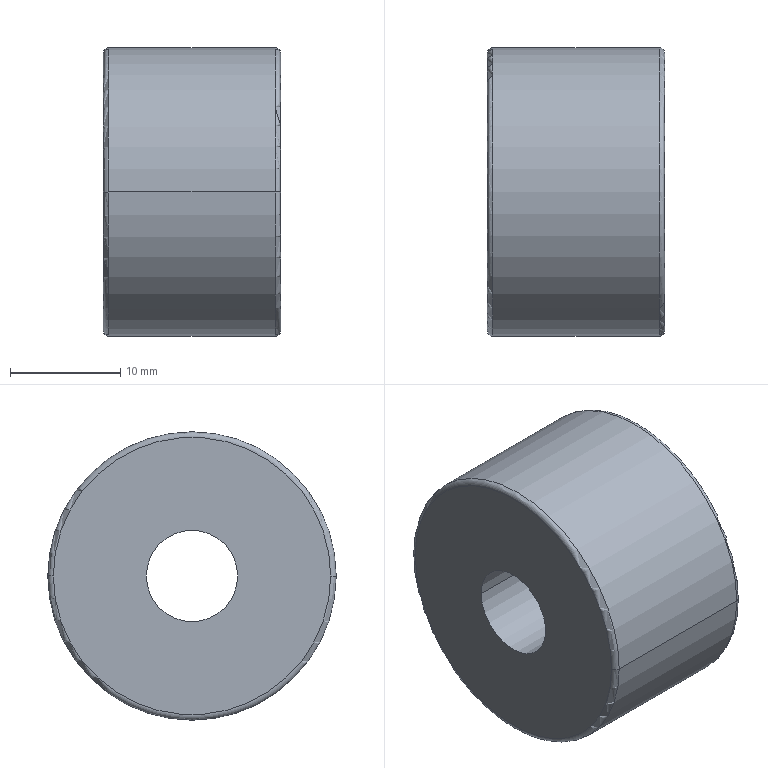Part | STEP file | 8XS224021_8GD.211.061 | 1 solid | 10 faces | box 16.1 x 26.2 x 26.2 mm | volume 7800 mm3 | torus 4 | cylinder 4 | plane 2 | commonest cylinder face diameters 8.3 x2 26.2 x2
STEP:
#1=CARTESIAN_POINT('',(0.,0.,0.));
#2=DIRECTION('',(0.,0.,1.));
#3=DIRECTION('',(1.,0.,0.));
#4=AXIS2_PLACEMENT_3D('',#1,#2,#3);
#5=CARTESIAN_POINT('',(5.5,-13.1,0.));
#6=VERTEX_POINT('',#5);
#7=CARTESIAN_POINT('',(5.5,13.1,0.));
#8=VERTEX_POINT('',#7);
#9=CARTESIAN_POINT('',(5.5,0.,0.));
#10=DIRECTION('',(-1.,0.,0.));
#11=DIRECTION('',(0.,1.,0.));
#12=AXIS2_PLACEMENT_3D('',#9,#10,#11);
#13=CIRCLE('',#12,13.1);
#14=CARTESIAN_POINT('',(5.5,0.,0.));
#15=DIRECTION('',(1.,0.,0.));
#16=DIRECTION('',(0.,1.,0.));
#17=AXIS2_PLACEMENT_3D('',#14,#15,#16);
#18=TOROIDAL_SURFACE('',#17,12.6,0.5);
#19=CARTESIAN_POINT('',(6.283,0.));
#20=DIRECTION('',(-1.,0.));
#21=VECTOR('',#20,1.);
#22=LINE('',#19,#21);
#23=(GEOMETRIC_REPRESENTATION_CONTEXT(2)PARAMETRIC_REPRESENTATION_CONTEXT()REPRESENTATION_CONTEXT('',''));
#24=DEFINITIONAL_REPRESENTATION('',(#22),#23);
#25=PCURVE('',#18,#24);
#26=CARTESIAN_POINT('',(6.,0.,0.));
#27=DIRECTION('',(1.,0.,0.));
#28=DIRECTION('',(0.,1.,0.));
#29=AXIS2_PLACEMENT_3D('',#26,#27,#28);
#30=CYLINDRICAL_SURFACE('',#29,13.1);
#31=CARTESIAN_POINT('',(6.283,-0.5));
#32=DIRECTION('',(-1.,0.));
#33=VECTOR('',#32,1.);
#34=LINE('',#31,#33);
#35=(GEOMETRIC_REPRESENTATION_CONTEXT(2)PARAMETRIC_REPRESENTATION_CONTEXT()REPRESENTATION_CONTEXT('',''));
#36=DEFINITIONAL_REPRESENTATION('',(#34),#35);
#37=PCURVE('',#30,#36);
#38=SURFACE_CURVE('',#13,(#25,#37),.PCURVE_S1.);
#39=EDGE_CURVE('',#6,#8,#38,.T.);
#40=ORIENTED_EDGE('',*,*,#39,.F.);
#41=CARTESIAN_POINT('',(6.,-12.6,0.));
#42=VERTEX_POINT('',#41);
#43=CARTESIAN_POINT('',(5.5,-12.6,0.));
#44=DIRECTION('',(0.,0.,1.));
#45=DIRECTION('',(0.,-1.,0.));
#46=AXIS2_PLACEMENT_3D('',#43,#44,#45);
#47=CIRCLE('',#46,0.5);
#48=CARTESIAN_POINT('',(3.142,0.));
#49=DIRECTION('',(0.,1.));
#50=VECTOR('',#49,1.);
#51=LINE('',#48,#50);
#52=(GEOMETRIC_REPRESENTATION_CONTEXT(2)PARAMETRIC_REPRESENTATION_CONTEXT()REPRESENTATION_CONTEXT('',''));
#53=DEFINITIONAL_REPRESENTATION('',(#51),#52);
#54=PCURVE('',#18,#53);
#55=CARTESIAN_POINT('',(5.5,0.,0.));
#56=DIRECTION('',(1.,0.,0.));
#57=DIRECTION('',(0.,1.,0.));
#58=AXIS2_PLACEMENT_3D('',#55,#56,#57);
#59=TOROIDAL_SURFACE('',#58,12.6,0.5);
#60=CARTESIAN_POINT('',(3.142,0.));
#61=DIRECTION('',(0.,1.));
#62=VECTOR('',#61,1.);
#63=LINE('',#60,#62);
#64=(GEOMETRIC_REPRESENTATION_CONTEXT(2)PARAMETRIC_REPRESENTATION_CONTEXT()REPRESENTATION_CONTEXT('',''));
#65=DEFINITIONAL_REPRESENTATION('',(#63),#64);
#66=PCURVE('',#59,#65);
#67=SURFACE_CURVE('',#47,(#54,#66),.PCURVE_S1.);
#68=EDGE_CURVE('',#6,#42,#67,.T.);
#69=ORIENTED_EDGE('',*,*,#68,.T.);
#70=CARTESIAN_POINT('',(6.,12.6,0.));
#71=VERTEX_POINT('',#70);
#72=CARTESIAN_POINT('',(6.,0.,0.));
#73=DIRECTION('',(1.,0.,0.));
#74=DIRECTION('',(0.,1.,0.));
#75=AXIS2_PLACEMENT_3D('',#72,#73,#74);
#76=CIRCLE('',#75,12.6);
#77=CARTESIAN_POINT('',(0.,1.571));
#78=DIRECTION('',(1.,0.));
#79=VECTOR('',#78,1.);
#80=LINE('',#77,#79);
#81=(GEOMETRIC_REPRESENTATION_CONTEXT(2)PARAMETRIC_REPRESENTATION_CONTEXT()REPRESENTATION_CONTEXT('',''));
#82=DEFINITIONAL_REPRESENTATION('',(#80),#81);
#83=PCURVE('',#18,#82);
#84=CARTESIAN_POINT('',(6.,13.1,0.));
#85=DIRECTION('',(1.,0.,0.));
#86=DIRECTION('',(0.,1.,0.));
#87=AXIS2_PLACEMENT_3D('',#84,#85,#86);
#88=PLANE('',#87);
#89=CARTESIAN_POINT('',(-13.1,0.));
#90=DIRECTION('',(1.,0.));
#91=AXIS2_PLACEMENT_2D('',#89,#90);
#92=CIRCLE('',#91,12.6);
#93=(GEOMETRIC_REPRESENTATION_CONTEXT(2)PARAMETRIC_REPRESENTATION_CONTEXT()REPRESENTATION_CONTEXT('',''));
#94=DEFINITIONAL_REPRESENTATION('',(#92),#93);
#95=PCURVE('',#88,#94);
#96=SURFACE_CURVE('',#76,(#83,#95),.PCURVE_S1.);
#97=EDGE_CURVE('',#71,#42,#96,.T.);
#98=ORIENTED_EDGE('',*,*,#97,.F.);
#99=CARTESIAN_POINT('',(5.5,12.6,0.));
#100=DIRECTION('',(0.,0.,-1.));
#101=DIRECTION('',(-1.,0.,0.));
#102=AXIS2_PLACEMENT_3D('',#99,#100,#101);
#103=CIRCLE('',#102,0.5);
#104=CARTESIAN_POINT('',(0.,-1.571));
#105=DIRECTION('',(0.,1.));
#106=VECTOR('',#105,1.);
#107=LINE('',#104,#106);
#108=(GEOMETRIC_REPRESENTATION_CONTEXT(2)PARAMETRIC_REPRESENTATION_CONTEXT()REPRESENTATION_CONTEXT('',''));
#109=DEFINITIONAL_REPRESENTATION('',(#107),#108);
#110=PCURVE('',#18,#109);
#111=CARTESIAN_POINT('',(6.283,-1.571));
#112=DIRECTION('',(0.,1.));
#113=VECTOR('',#112,1.);
#114=LINE('',#111,#113);
#115=(GEOMETRIC_REPRESENTATION_CONTEXT(2)PARAMETRIC_REPRESENTATION_CONTEXT()REPRESENTATION_CONTEXT('',''));
#116=DEFINITIONAL_REPRESENTATION('',(#114),#115);
#117=PCURVE('',#59,#116);
#118=SURFACE_CURVE('',#103,(#110,#117),.PCURVE_S1.);
#119=EDGE_CURVE('',#8,#71,#118,.T.);
#120=ORIENTED_EDGE('',*,*,#119,.F.);
#121=EDGE_LOOP('',(#40,#69,#98,#120));
#122=FACE_BOUND('',#121,.T.);
#123=ADVANCED_FACE('',(#122),#18,.T.);
#124=CARTESIAN_POINT('',(-9.6,13.1,0.));
#125=VERTEX_POINT('',#124);
#126=CARTESIAN_POINT('',(-9.6,-13.1,0.));
#127=VERTEX_POINT('',#126);
#128=CARTESIAN_POINT('',(-9.6,0.,0.));
#129=DIRECTION('',(1.,0.,0.));
#130=DIRECTION('',(0.,-1.,0.));
#131=AXIS2_PLACEMENT_3D('',#128,#129,#130);
#132=CIRCLE('',#131,13.1);
#133=CARTESIAN_POINT('',(-9.6,0.,0.));
#134=DIRECTION('',(-1.,0.,0.));
#135=DIRECTION('',(0.,-1.,0.));
#136=AXIS2_PLACEMENT_3D('',#133,#134,#135);
#137=TOROIDAL_SURFACE('',#136,12.6,0.5);
#138=CARTESIAN_POINT('',(6.283,0.));
#139=DIRECTION('',(-1.,0.));
#140=VECTOR('',#139,1.);
#141=LINE('',#138,#140);
#142=(GEOMETRIC_REPRESENTATION_CONTEXT(2)PARAMETRIC_REPRESENTATION_CONTEXT()REPRESENTATION_CONTEXT('',''));
#143=DEFINITIONAL_REPRESENTATION('',(#141),#142);
#144=PCURVE('',#137,#143);
#145=CARTESIAN_POINT('',(-3.142,-15.6));
#146=DIRECTION('',(1.,0.));
#147=VECTOR('',#146,1.);
#148=LINE('',#145,#147);
#149=(GEOMETRIC_REPRESENTATION_CONTEXT(2)PARAMETRIC_REPRESENTATION_CONTEXT()REPRESENTATION_CONTEXT('',''));
#150=DEFINITIONAL_REPRESENTATION('',(#148),#149);
#151=PCURVE('',#30,#150);
#152=SURFACE_CURVE('',#132,(#144,#151),.PCURVE_S1.);
#153=EDGE_CURVE('',#125,#127,#152,.T.);
#154=ORIENTED_EDGE('',*,*,#153,.F.);
#155=CARTESIAN_POINT('',(-10.1,12.6,0.));
#156=VERTEX_POINT('',#155);
#157=CARTESIAN_POINT('',(-9.6,12.6,0.));
#158=DIRECTION('',(0.,0.,1.));
#159=DIRECTION('',(0.,-1.,0.));
#160=AXIS2_PLACEMENT_3D('',#157,#158,#159);
#161=CIRCLE('',#160,0.5);
#162=CARTESIAN_POINT('',(3.142,-3.142));
#163=DIRECTION('',(0.,1.));
#164=VECTOR('',#163,1.);
#165=LINE('',#162,#164);
#166=(GEOMETRIC_REPRESENTATION_CONTEXT(2)PARAMETRIC_REPRESENTATION_CONTEXT()REPRESENTATION_CONTEXT('',''));
#167=DEFINITIONAL_REPRESENTATION('',(#165),#166);
#168=PCURVE('',#137,#167);
#169=CARTESIAN_POINT('',(-9.6,0.,0.));
#170=DIRECTION('',(-1.,0.,0.));
#171=DIRECTION('',(0.,-1.,0.));
#172=AXIS2_PLACEMENT_3D('',#169,#170,#171);
#173=TOROIDAL_SURFACE('',#172,12.6,0.5);
#174=CARTESIAN_POINT('',(3.142,-3.142));
#175=DIRECTION('',(0.,1.));
#176=VECTOR('',#175,1.);
#177=LINE('',#174,#176);
#178=(GEOMETRIC_REPRESENTATION_CONTEXT(2)PARAMETRIC_REPRESENTATION_CONTEXT()REPRESENTATION_CONTEXT('',''));
#179=DEFINITIONAL_REPRESENTATION('',(#177),#178);
#180=PCURVE('',#173,#179);
#181=SURFACE_CURVE('',#161,(#168,#180),.PCURVE_S1.);
#182=EDGE_CURVE('',#125,#156,#181,.T.);
#183=ORIENTED_EDGE('',*,*,#182,.T.);
#184=CARTESIAN_POINT('',(-10.1,-12.6,0.));
#185=VERTEX_POINT('',#184);
#186=CARTESIAN_POINT('',(-10.1,0.,0.));
#187=DIRECTION('',(-1.,0.,0.));
#188=DIRECTION('',(0.,-1.,0.));
#189=AXIS2_PLACEMENT_3D('',#186,#187,#188);
#190=CIRCLE('',#189,12.6);
#191=CARTESIAN_POINT('',(0.,1.571));
#192=DIRECTION('',(1.,0.));
#193=VECTOR('',#192,1.);
#194=LINE('',#191,#193);
#195=(GEOMETRIC_REPRESENTATION_CONTEXT(2)PARAMETRIC_REPRESENTATION_CONTEXT()REPRESENTATION_CONTEXT('',''));
#196=DEFINITIONAL_REPRESENTATION('',(#194),#195);
#197=PCURVE('',#137,#196);
#198=CARTESIAN_POINT('',(-10.1,13.1,0.));
#199=DIRECTION('',(-1.,0.,0.));
#200=DIRECTION('',(0.,-1.,0.));
#201=AXIS2_PLACEMENT_3D('',#198,#199,#200);
#202=PLANE('',#201);
#203=CARTESIAN_POINT('',(13.1,0.));
#204=DIRECTION('',(1.,0.));
#205=AXIS2_PLACEMENT_2D('',#203,#204);
#206=CIRCLE('',#205,12.6);
#207=(GEOMETRIC_REPRESENTATION_CONTEXT(2)PARAMETRIC_REPRESENTATION_CONTEXT()REPRESENTATION_CONTEXT('',''));
#208=DEFINITIONAL_REPRESENTATION('',(#206),#207);
#209=PCURVE('',#202,#208);
#210=SURFACE_CURVE('',#190,(#197,#209),.PCURVE_S1.);
#211=EDGE_CURVE('',#185,#156,#210,.T.);
#212=ORIENTED_EDGE('',*,*,#211,.F.);
#213=CARTESIAN_POINT('',(-9.6,-12.6,0.));
#214=DIRECTION('',(0.,0.,-1.));
#215=DIRECTION('',(-1.,0.,0.));
#216=AXIS2_PLACEMENT_3D('',#213,#214,#215);
#217=CIRCLE('',#216,0.5);
#218=CARTESIAN_POINT('',(0.,-4.712));
#219=DIRECTION('',(0.,1.));
#220=VECTOR('',#219,1.);
#221=LINE('',#218,#220);
#222=(GEOMETRIC_REPRESENTATION_CONTEXT(2)PARAMETRIC_REPRESENTATION_CONTEXT()REPRESENTATION_CONTEXT('',''));
#223=DEFINITIONAL_REPRESENTATION('',(#221),#222);
#224=PCURVE('',#137,#223);
#225=CARTESIAN_POINT('',(6.283,-4.712));
#226=DIRECTION('',(0.,1.));
#227=VECTOR('',#226,1.);
#228=LINE('',#225,#227);
#229=(GEOMETRIC_REPRESENTATION_CONTEXT(2)PARAMETRIC_REPRESENTATION_CONTEXT()REPRESENTATION_CONTEXT('',''));
#230=DEFINITIONAL_REPRESENTATION('',(#228),#229);
#231=PCURVE('',#173,#230);
#232=SURFACE_CURVE('',#217,(#224,#231),.PCURVE_S1.);
#233=EDGE_CURVE('',#127,#185,#232,.T.);
#234=ORIENTED_EDGE('',*,*,#233,.F.);
#235=EDGE_LOOP('',(#154,#183,#212,#234));
#236=FACE_BOUND('',#235,.T.);
#237=ADVANCED_FACE('',(#236),#137,.T.);
#238=ORIENTED_EDGE('',*,*,#153,.T.);
#239=CARTESIAN_POINT('',(6.,-13.1,0.));
#240=DIRECTION('',(1.,0.,0.));
#241=VECTOR('',#240,1.);
#242=LINE('',#239,#241);
#243=CARTESIAN_POINT('',(3.142,0.));
#244=DIRECTION('',(0.,1.));
#245=VECTOR('',#244,1.);
#246=LINE('',#243,#245);
#247=(GEOMETRIC_REPRESENTATION_CONTEXT(2)PARAMETRIC_REPRESENTATION_CONTEXT()REPRESENTATION_CONTEXT('',''));
#248=DEFINITIONAL_REPRESENTATION('',(#246),#247);
#249=PCURVE('',#30,#248);
#250=CARTESIAN_POINT('',(6.,0.,0.));
#251=DIRECTION('',(1.,0.,0.));
#252=DIRECTION('',(0.,1.,0.));
#253=AXIS2_PLACEMENT_3D('',#250,#251,#252);
#254=CYLINDRICAL_SURFACE('',#253,13.1);
#255=CARTESIAN_POINT('',(3.142,0.));
#256=DIRECTION('',(0.,1.));
#257=VECTOR('',#256,1.);
#258=LINE('',#255,#257);
#259=(GEOMETRIC_REPRESENTATION_CONTEXT(2)PARAMETRIC_REPRESENTATION_CONTEXT()REPRESENTATION_CONTEXT('',''));
#260=DEFINITIONAL_REPRESENTATION('',(#258),#259);
#261=PCURVE('',#254,#260);
#262=SURFACE_CURVE('',#242,(#249,#261),.PCURVE_S1.);
#263=EDGE_CURVE('',#127,#6,#262,.T.);
#264=ORIENTED_EDGE('',*,*,#263,.T.);
#265=ORIENTED_EDGE('',*,*,#39,.T.);
#266=CARTESIAN_POINT('',(6.,13.1,0.));
#267=DIRECTION('',(1.,0.,0.));
#268=VECTOR('',#267,1.);
#269=LINE('',#266,#268);
#270=CARTESIAN_POINT('',(0.,0.));
#271=DIRECTION('',(0.,1.));
#272=VECTOR('',#271,1.);
#273=LINE('',#270,#272);
#274=(GEOMETRIC_REPRESENTATION_CONTEXT(2)PARAMETRIC_REPRESENTATION_CONTEXT()REPRESENTATION_CONTEXT('',''));
#275=DEFINITIONAL_REPRESENTATION('',(#273),#274);
#276=PCURVE('',#30,#275);
#277=CARTESIAN_POINT('',(6.283,0.));
#278=DIRECTION('',(0.,1.));
#279=VECTOR('',#278,1.);
#280=LINE('',#277,#279);
#281=(GEOMETRIC_REPRESENTATION_CONTEXT(2)PARAMETRIC_REPRESENTATION_CONTEXT()REPRESENTATION_CONTEXT('',''));
#282=DEFINITIONAL_REPRESENTATION('',(#280),#281);
#283=PCURVE('',#254,#282);
#284=SURFACE_CURVE('',#269,(#276,#283),.PCURVE_S1.);
#285=EDGE_CURVE('',#125,#8,#284,.T.);
#286=ORIENTED_EDGE('',*,*,#285,.F.);
#287=EDGE_LOOP('',(#238,#264,#265,#286));
#288=FACE_BOUND('',#287,.T.);
#289=ADVANCED_FACE('',(#288),#30,.T.);
#290=CARTESIAN_POINT('',(-10.1,4.15,0.));
#291=VERTEX_POINT('',#290);
#292=CARTESIAN_POINT('',(6.,4.15,0.));
#293=VERTEX_POINT('',#292);
#294=CARTESIAN_POINT('',(6.,4.15,0.));
#295=DIRECTION('',(1.,0.,0.));
#296=VECTOR('',#295,1.);
#297=LINE('',#294,#296);
#298=CARTESIAN_POINT('',(6.,0.,0.));
#299=DIRECTION('',(1.,0.,0.));
#300=DIRECTION('',(0.,1.,0.));
#301=AXIS2_PLACEMENT_3D('',#298,#299,#300);
#302=CYLINDRICAL_SURFACE('',#301,4.15);
#303=CARTESIAN_POINT('',(6.283,0.));
#304=DIRECTION('',(0.,1.));
#305=VECTOR('',#304,1.);
#306=LINE('',#303,#305);
#307=(GEOMETRIC_REPRESENTATION_CONTEXT(2)PARAMETRIC_REPRESENTATION_CONTEXT()REPRESENTATION_CONTEXT('',''));
#308=DEFINITIONAL_REPRESENTATION('',(#306),#307);
#309=PCURVE('',#302,#308);
#310=CARTESIAN_POINT('',(6.,0.,0.));
#311=DIRECTION('',(1.,0.,0.));
#312=DIRECTION('',(0.,1.,0.));
#313=AXIS2_PLACEMENT_3D('',#310,#311,#312);
#314=CYLINDRICAL_SURFACE('',#313,4.15);
#315=CARTESIAN_POINT('',(0.,0.));
#316=DIRECTION('',(0.,1.));
#317=VECTOR('',#316,1.);
#318=LINE('',#315,#317);
#319=(GEOMETRIC_REPRESENTATION_CONTEXT(2)PARAMETRIC_REPRESENTATION_CONTEXT()REPRESENTATION_CONTEXT('',''));
#320=DEFINITIONAL_REPRESENTATION('',(#318),#319);
#321=PCURVE('',#314,#320);
#322=SURFACE_CURVE('',#297,(#309,#321),.PCURVE_S1.);
#323=EDGE_CURVE('',#291,#293,#322,.T.);
#324=ORIENTED_EDGE('',*,*,#323,.T.);
#325=CARTESIAN_POINT('',(6.,-4.15,0.));
#326=VERTEX_POINT('',#325);
#327=CARTESIAN_POINT('',(6.,0.,0.));
#328=DIRECTION('',(1.,0.,0.));
#329=DIRECTION('',(0.,1.,0.));
#330=AXIS2_PLACEMENT_3D('',#327,#328,#329);
#331=CIRCLE('',#330,4.15);
#332=CARTESIAN_POINT('',(0.,0.));
#333=DIRECTION('',(1.,0.));
#334=VECTOR('',#333,1.);
#335=LINE('',#332,#334);
#336=(GEOMETRIC_REPRESENTATION_CONTEXT(2)PARAMETRIC_REPRESENTATION_CONTEXT()REPRESENTATION_CONTEXT('',''));
#337=DEFINITIONAL_REPRESENTATION('',(#335),#336);
#338=PCURVE('',#302,#337);
#339=CARTESIAN_POINT('',(-13.1,0.));
#340=DIRECTION('',(1.,0.));
#341=AXIS2_PLACEMENT_2D('',#339,#340);
#342=CIRCLE('',#341,4.15);
#343=(GEOMETRIC_REPRESENTATION_CONTEXT(2)PARAMETRIC_REPRESENTATION_CONTEXT()REPRESENTATION_CONTEXT('',''));
#344=DEFINITIONAL_REPRESENTATION('',(#342),#343);
#345=PCURVE('',#88,#344);
#346=SURFACE_CURVE('',#331,(#338,#345),.PCURVE_S1.);
#347=EDGE_CURVE('',#326,#293,#346,.T.);
#348=ORIENTED_EDGE('',*,*,#347,.F.);
#349=CARTESIAN_POINT('',(-10.1,-4.15,0.));
#350=VERTEX_POINT('',#349);
#351=CARTESIAN_POINT('',(6.,-4.15,0.));
#352=DIRECTION('',(1.,0.,0.));
#353=VECTOR('',#352,1.);
#354=LINE('',#351,#353);
#355=CARTESIAN_POINT('',(3.142,0.));
#356=DIRECTION('',(0.,1.));
#357=VECTOR('',#356,1.);
#358=LINE('',#355,#357);
#359=(GEOMETRIC_REPRESENTATION_CONTEXT(2)PARAMETRIC_REPRESENTATION_CONTEXT()REPRESENTATION_CONTEXT('',''));
#360=DEFINITIONAL_REPRESENTATION('',(#358),#359);
#361=PCURVE('',#302,#360);
#362=CARTESIAN_POINT('',(3.142,0.));
#363=DIRECTION('',(0.,1.));
#364=VECTOR('',#363,1.);
#365=LINE('',#362,#364);
#366=(GEOMETRIC_REPRESENTATION_CONTEXT(2)PARAMETRIC_REPRESENTATION_CONTEXT()REPRESENTATION_CONTEXT('',''));
#367=DEFINITIONAL_REPRESENTATION('',(#365),#366);
#368=PCURVE('',#314,#367);
#369=SURFACE_CURVE('',#354,(#361,#368),.PCURVE_S1.);
#370=EDGE_CURVE('',#350,#326,#369,.T.);
#371=ORIENTED_EDGE('',*,*,#370,.F.);
#372=CARTESIAN_POINT('',(-10.1,0.,0.));
#373=DIRECTION('',(1.,0.,0.));
#374=DIRECTION('',(0.,1.,0.));
#375=AXIS2_PLACEMENT_3D('',#372,#373,#374);
#376=CIRCLE('',#375,4.15);
#377=CARTESIAN_POINT('',(0.,-16.1));
#378=DIRECTION('',(1.,0.));
#379=VECTOR('',#378,1.);
#380=LINE('',#377,#379);
#381=(GEOMETRIC_REPRESENTATION_CONTEXT(2)PARAMETRIC_REPRESENTATION_CONTEXT()REPRESENTATION_CONTEXT('',''));
#382=DEFINITIONAL_REPRESENTATION('',(#380),#381);
#383=PCURVE('',#302,#382);
#384=CARTESIAN_POINT('',(8.95,0.));
#385=CARTESIAN_POINT('',(8.95,7.188));
#386=CARTESIAN_POINT('',(15.175,3.594));
#387=CARTESIAN_POINT('',(21.4,0.));
#388=CARTESIAN_POINT('',(15.175,-3.594));
#389=CARTESIAN_POINT('',(8.95,-7.188));
#390=CARTESIAN_POINT('',(8.95,0.));
#391=(BOUNDED_CURVE()B_SPLINE_CURVE(2,(#384,#385,#386,#387,#388,#389,#390),.UNSPECIFIED.,.T.,.F.)B_SPLINE_CURVE_WITH_KNOTS((1,2,2,2,2,1),(-2.094,0.,2.094,4.189,6.283,8.378),.UNSPECIFIED.)CURVE()GEOMETRIC_REPRESENTATION_ITEM()RATIONAL_B_SPLINE_CURVE((1.,0.5,1.,0.5,1.,0.5,1.))REPRESENTATION_ITEM(''));
#392=(GEOMETRIC_REPRESENTATION_CONTEXT(2)PARAMETRIC_REPRESENTATION_CONTEXT()REPRESENTATION_CONTEXT('',''));
#393=DEFINITIONAL_REPRESENTATION('',(#391),#392);
#394=PCURVE('',#202,#393);
#395=SURFACE_CURVE('',#376,(#383,#394),.PCURVE_S1.);
#396=EDGE_CURVE('',#350,#291,#395,.T.);
#397=ORIENTED_EDGE('',*,*,#396,.T.);
#398=EDGE_LOOP('',(#324,#348,#371,#397));
#399=FACE_BOUND('',#398,.F.);
#400=ADVANCED_FACE('',(#399),#302,.F.);
#401=CARTESIAN_POINT('',(6.,0.,0.));
#402=DIRECTION('',(1.,0.,0.));
#403=DIRECTION('',(0.,1.,0.));
#404=AXIS2_PLACEMENT_3D('',#401,#402,#403);
#405=CIRCLE('',#404,4.15);
#406=CARTESIAN_POINT('',(0.,0.));
#407=DIRECTION('',(1.,0.));
#408=VECTOR('',#407,1.);
#409=LINE('',#406,#408);
#410=(GEOMETRIC_REPRESENTATION_CONTEXT(2)PARAMETRIC_REPRESENTATION_CONTEXT()REPRESENTATION_CONTEXT('',''));
#411=DEFINITIONAL_REPRESENTATION('',(#409),#410);
#412=PCURVE('',#314,#411);
#413=CARTESIAN_POINT('',(-13.1,0.));
#414=DIRECTION('',(1.,0.));
#415=AXIS2_PLACEMENT_2D('',#413,#414);
#416=CIRCLE('',#415,4.15);
#417=(GEOMETRIC_REPRESENTATION_CONTEXT(2)PARAMETRIC_REPRESENTATION_CONTEXT()REPRESENTATION_CONTEXT('',''));
#418=DEFINITIONAL_REPRESENTATION('',(#416),#417);
#419=PCURVE('',#88,#418);
#420=SURFACE_CURVE('',#405,(#412,#419),.PCURVE_S1.);
#421=EDGE_CURVE('',#293,#326,#420,.T.);
#422=ORIENTED_EDGE('',*,*,#421,.F.);
#423=ORIENTED_EDGE('',*,*,#323,.F.);
#424=CARTESIAN_POINT('',(-10.1,0.,0.));
#425=DIRECTION('',(1.,0.,0.));
#426=DIRECTION('',(0.,1.,0.));
#427=AXIS2_PLACEMENT_3D('',#424,#425,#426);
#428=CIRCLE('',#427,4.15);
#429=CARTESIAN_POINT('',(0.,-16.1));
#430=DIRECTION('',(1.,0.));
#431=VECTOR('',#430,1.);
#432=LINE('',#429,#431);
#433=(GEOMETRIC_REPRESENTATION_CONTEXT(2)PARAMETRIC_REPRESENTATION_CONTEXT()REPRESENTATION_CONTEXT('',''));
#434=DEFINITIONAL_REPRESENTATION('',(#432),#433);
#435=PCURVE('',#314,#434);
#436=CARTESIAN_POINT('',(8.95,0.));
#437=CARTESIAN_POINT('',(8.95,7.188));
#438=CARTESIAN_POINT('',(15.175,3.594));
#439=CARTESIAN_POINT('',(21.4,0.));
#440=CARTESIAN_POINT('',(15.175,-3.594));
#441=CARTESIAN_POINT('',(8.95,-7.188));
#442=CARTESIAN_POINT('',(8.95,0.));
#443=(BOUNDED_CURVE()B_SPLINE_CURVE(2,(#436,#437,#438,#439,#440,#441,#442),.UNSPECIFIED.,.T.,.F.)B_SPLINE_CURVE_WITH_KNOTS((1,2,2,2,2,1),(-2.094,0.,2.094,4.189,6.283,8.378),.UNSPECIFIED.)CURVE()GEOMETRIC_REPRESENTATION_ITEM()RATIONAL_B_SPLINE_CURVE((1.,0.5,1.,0.5,1.,0.5,1.))REPRESENTATION_ITEM(''));
#444=(GEOMETRIC_REPRESENTATION_CONTEXT(2)PARAMETRIC_REPRESENTATION_CONTEXT()REPRESENTATION_CONTEXT('',''));
#445=DEFINITIONAL_REPRESENTATION('',(#443),#444);
#446=PCURVE('',#202,#445);
#447=SURFACE_CURVE('',#428,(#435,#446),.PCURVE_S1.);
#448=EDGE_CURVE('',#291,#350,#447,.T.);
#449=ORIENTED_EDGE('',*,*,#448,.T.);
#450=ORIENTED_EDGE('',*,*,#370,.T.);
#451=EDGE_LOOP('',(#422,#423,#449,#450));
#452=FACE_BOUND('',#451,.F.);
#453=ADVANCED_FACE('',(#452),#314,.F.);
#454=ORIENTED_EDGE('',*,*,#211,.T.);
#455=CARTESIAN_POINT('',(-10.1,0.,0.));
#456=DIRECTION('',(-1.,0.,0.));
#457=DIRECTION('',(0.,-1.,0.));
#458=AXIS2_PLACEMENT_3D('',#455,#456,#457);
#459=CIRCLE('',#458,12.6);
#460=CARTESIAN_POINT('',(13.1,0.));
#461=DIRECTION('',(1.,0.));
#462=AXIS2_PLACEMENT_2D('',#460,#461);
#463=CIRCLE('',#462,12.6);
#464=(GEOMETRIC_REPRESENTATION_CONTEXT(2)PARAMETRIC_REPRESENTATION_CONTEXT()REPRESENTATION_CONTEXT('',''));
#465=DEFINITIONAL_REPRESENTATION('',(#463),#464);
#466=PCURVE('',#202,#465);
#467=CARTESIAN_POINT('',(0.,1.571));
#468=DIRECTION('',(1.,0.));
#469=VECTOR('',#468,1.);
#470=LINE('',#467,#469);
#471=(GEOMETRIC_REPRESENTATION_CONTEXT(2)PARAMETRIC_REPRESENTATION_CONTEXT()REPRESENTATION_CONTEXT('',''));
#472=DEFINITIONAL_REPRESENTATION('',(#470),#471);
#473=PCURVE('',#173,#472);
#474=SURFACE_CURVE('',#459,(#466,#473),.PCURVE_S1.);
#475=EDGE_CURVE('',#156,#185,#474,.T.);
#476=ORIENTED_EDGE('',*,*,#475,.T.);
#477=EDGE_LOOP('',(#454,#476));
#478=FACE_BOUND('',#477,.T.);
#479=ORIENTED_EDGE('',*,*,#448,.T.);
#480=ORIENTED_EDGE('',*,*,#396,.T.);
#481=EDGE_LOOP('',(#479,#480));
#482=FACE_BOUND('',#481,.T.);
#483=ADVANCED_FACE('',(#478,#482),#202,.T.);
#484=ORIENTED_EDGE('',*,*,#263,.F.);
#485=CARTESIAN_POINT('',(-9.6,0.,0.));
#486=DIRECTION('',(1.,0.,0.));
#487=DIRECTION('',(0.,-1.,0.));
#488=AXIS2_PLACEMENT_3D('',#485,#486,#487);
#489=CIRCLE('',#488,13.1);
#490=CARTESIAN_POINT('',(3.142,-15.6));
#491=DIRECTION('',(1.,0.));
#492=VECTOR('',#491,1.);
#493=LINE('',#490,#492);
#494=(GEOMETRIC_REPRESENTATION_CONTEXT(2)PARAMETRIC_REPRESENTATION_CONTEXT()REPRESENTATION_CONTEXT('',''));
#495=DEFINITIONAL_REPRESENTATION('',(#493),#494);
#496=PCURVE('',#254,#495);
#497=CARTESIAN_POINT('',(6.283,0.));
#498=DIRECTION('',(-1.,0.));
#499=VECTOR('',#498,1.);
#500=LINE('',#497,#499);
#501=(GEOMETRIC_REPRESENTATION_CONTEXT(2)PARAMETRIC_REPRESENTATION_CONTEXT()REPRESENTATION_CONTEXT('',''));
#502=DEFINITIONAL_REPRESENTATION('',(#500),#501);
#503=PCURVE('',#173,#502);
#504=SURFACE_CURVE('',#489,(#496,#503),.PCURVE_S1.);
#505=EDGE_CURVE('',#127,#125,#504,.T.);
#506=ORIENTED_EDGE('',*,*,#505,.T.);
#507=ORIENTED_EDGE('',*,*,#285,.T.);
#508=CARTESIAN_POINT('',(5.5,0.,0.));
#509=DIRECTION('',(-1.,0.,0.));
#510=DIRECTION('',(0.,1.,0.));
#511=AXIS2_PLACEMENT_3D('',#508,#509,#510);
#512=CIRCLE('',#511,13.1);
#513=CARTESIAN_POINT('',(6.283,-0.5));
#514=DIRECTION('',(-1.,0.));
#515=VECTOR('',#514,1.);
#516=LINE('',#513,#515);
#517=(GEOMETRIC_REPRESENTATION_CONTEXT(2)PARAMETRIC_REPRESENTATION_CONTEXT()REPRESENTATION_CONTEXT('',''));
#518=DEFINITIONAL_REPRESENTATION('',(#516),#517);
#519=PCURVE('',#254,#518);
#520=CARTESIAN_POINT('',(6.283,0.));
#521=DIRECTION('',(-1.,0.));
#522=VECTOR('',#521,1.);
#523=LINE('',#520,#522);
#524=(GEOMETRIC_REPRESENTATION_CONTEXT(2)PARAMETRIC_REPRESENTATION_CONTEXT()REPRESENTATION_CONTEXT('',''));
#525=DEFINITIONAL_REPRESENTATION('',(#523),#524);
#526=PCURVE('',#59,#525);
#527=SURFACE_CURVE('',#512,(#519,#526),.PCURVE_S1.);
#528=EDGE_CURVE('',#8,#6,#527,.T.);
#529=ORIENTED_EDGE('',*,*,#528,.T.);
#530=EDGE_LOOP('',(#484,#506,#507,#529));
#531=FACE_BOUND('',#530,.T.);
#532=ADVANCED_FACE('',(#531),#254,.T.);
#533=ORIENTED_EDGE('',*,*,#97,.T.);
#534=CARTESIAN_POINT('',(6.,0.,0.));
#535=DIRECTION('',(1.,0.,0.));
#536=DIRECTION('',(0.,1.,0.));
#537=AXIS2_PLACEMENT_3D('',#534,#535,#536);
#538=CIRCLE('',#537,12.6);
#539=CARTESIAN_POINT('',(-13.1,0.));
#540=DIRECTION('',(1.,0.));
#541=AXIS2_PLACEMENT_2D('',#539,#540);
#542=CIRCLE('',#541,12.6);
#543=(GEOMETRIC_REPRESENTATION_CONTEXT(2)PARAMETRIC_REPRESENTATION_CONTEXT()REPRESENTATION_CONTEXT('',''));
#544=DEFINITIONAL_REPRESENTATION('',(#542),#543);
#545=PCURVE('',#88,#544);
#546=CARTESIAN_POINT('',(0.,1.571));
#547=DIRECTION('',(1.,0.));
#548=VECTOR('',#547,1.);
#549=LINE('',#546,#548);
#550=(GEOMETRIC_REPRESENTATION_CONTEXT(2)PARAMETRIC_REPRESENTATION_CONTEXT()REPRESENTATION_CONTEXT('',''));
#551=DEFINITIONAL_REPRESENTATION('',(#549),#550);
#552=PCURVE('',#59,#551);
#553=SURFACE_CURVE('',#538,(#545,#552),.PCURVE_S1.);
#554=EDGE_CURVE('',#42,#71,#553,.T.);
#555=ORIENTED_EDGE('',*,*,#554,.T.);
#556=EDGE_LOOP('',(#533,#555));
#557=FACE_BOUND('',#556,.T.);
#558=ORIENTED_EDGE('',*,*,#421,.F.);
#559=ORIENTED_EDGE('',*,*,#347,.F.);
#560=EDGE_LOOP('',(#558,#559));
#561=FACE_BOUND('',#560,.T.);
#562=ADVANCED_FACE('',(#557,#561),#88,.T.);
#563=ORIENTED_EDGE('',*,*,#182,.F.);
#564=ORIENTED_EDGE('',*,*,#505,.F.);
#565=ORIENTED_EDGE('',*,*,#233,.T.);
#566=ORIENTED_EDGE('',*,*,#475,.F.);
#567=EDGE_LOOP('',(#563,#564,#565,#566));
#568=FACE_BOUND('',#567,.T.);
#569=ADVANCED_FACE('',(#568),#173,.T.);
#570=ORIENTED_EDGE('',*,*,#68,.F.);
#571=ORIENTED_EDGE('',*,*,#528,.F.);
#572=ORIENTED_EDGE('',*,*,#119,.T.);
#573=ORIENTED_EDGE('',*,*,#554,.F.);
#574=EDGE_LOOP('',(#570,#571,#572,#573));
#575=FACE_BOUND('',#574,.T.);
#576=ADVANCED_FACE('',(#575),#59,.T.);
#577=CLOSED_SHELL('',(#123,#237,#289,#400,#453,#483,#532,#562,#569,#576));
#578=MANIFOLD_SOLID_BREP('',#577);
#579=(LENGTH_UNIT()NAMED_UNIT(*)SI_UNIT(.MILLI.,.METRE.));
#580=UNCERTAINTY_MEASURE_WITH_UNIT(LENGTH_MEASURE(0.0000001),#579,'','');
#581=(NAMED_UNIT(*)PLANE_ANGLE_UNIT()SI_UNIT($,.RADIAN.));
#582=(NAMED_UNIT(*)SI_UNIT($,.STERADIAN.)SOLID_ANGLE_UNIT());
#583=(GEOMETRIC_REPRESENTATION_CONTEXT(3)GLOBAL_UNCERTAINTY_ASSIGNED_CONTEXT((#580))GLOBAL_UNIT_ASSIGNED_CONTEXT((#579,#581,#582))REPRESENTATION_CONTEXT('',''));
#584=ADVANCED_BREP_SHAPE_REPRESENTATION('',(#4,#578),#583);